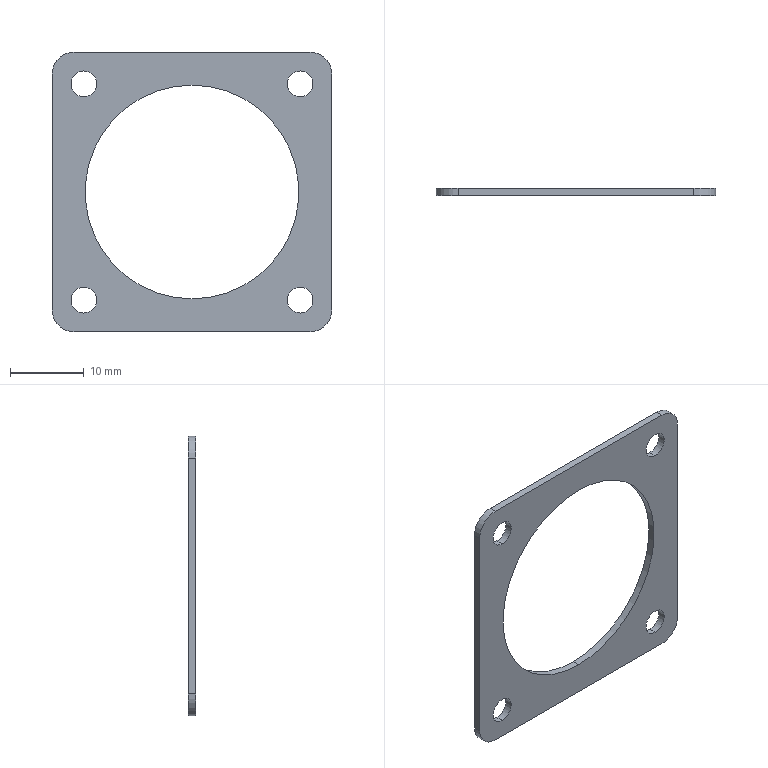Part | STEP file | 15050041--1-60790001 | 1 solid | 20 faces | box 38 x 1 x 38 mm | volume 737.27 mm3 | cylinder 14 | plane 6 | commonest cylinder face diameters 3.5 x8 6 x4 29 x2